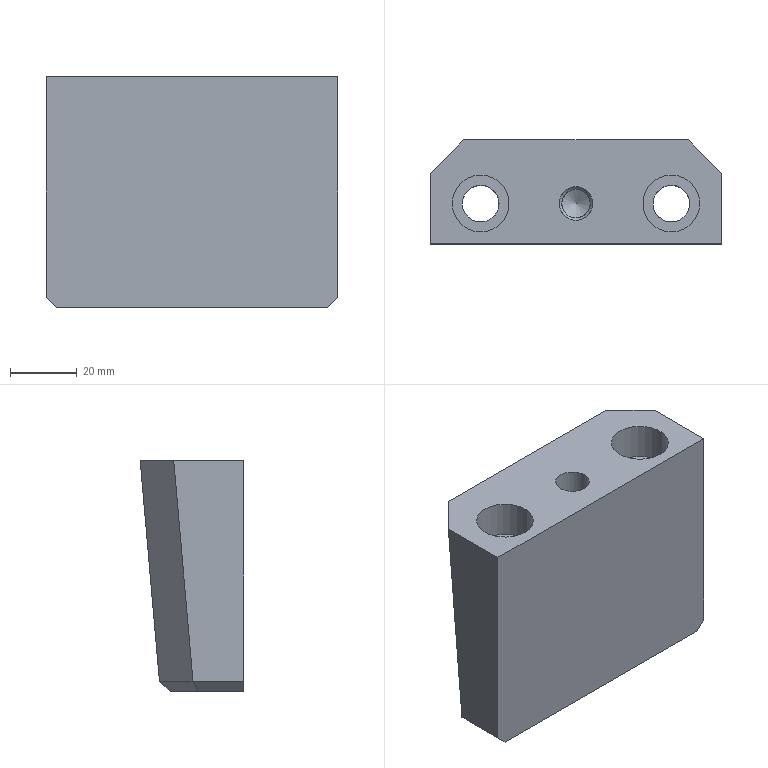Part | STEP file | P011002NM07-000 | 1 solid | 30 faces | box 87 x 31 x 69 mm | volume 142784 mm3 | plane 19 | cylinder 7 | cone 4 | commonest cylinder face diameters 11 x2 17 x2 8.5 x1 9.967 x1 10 x1